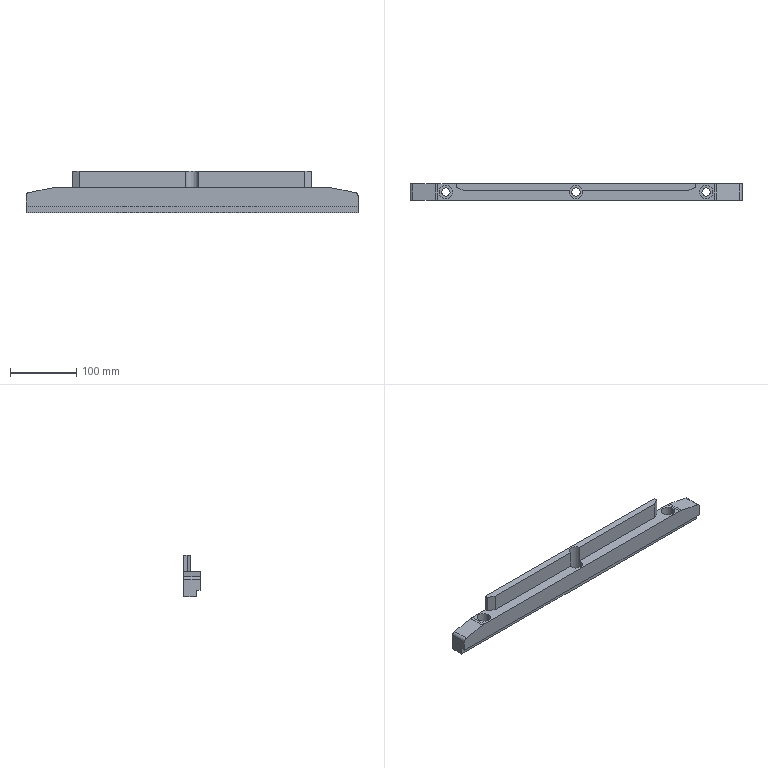NC program | NX | posted with a generic post | part box 500 x 25 x 62.5 mm
Lines 30 to 1063 of 3905:
(ADAPTIVE_MILLING_COPY , TOOL : D12JING)
N52 T21 M6
N54 G54
N56 G17 G0 G90 X258.765 Y-15.498 S9500 M3
N58 G43 Z30. H21
N60 Z-8.
N62 G94 G1 Z-9. F1000.
N64 X257.053 Y-13.023 F3000.
N66 G3 X256.056 Y-12.5 R1.229
N68 G2 X250.891 Y-16.168 R9.884
N70 X243.653 Y-17.311 R27.235
N72 X230.756 Y-17.483 R318.29
N74 G1 X225.881 Y-17.486
N76 X200.156 Y-17.487
N78 X50.756
N80 X50.081 Y-17.49
N82 X49.031 Y-17.492
N84 X48.581
N86 X47.681 Y-17.495
N88 X46.406 Y-17.493
N90 X45.581 Y-17.496
N92 X44.456 Y-17.495
N94 X43.631 Y-17.497
N96 X42.581 Y-17.496
N98 X41.681 Y-17.498
N100 X40.931 Y-17.497
N102 X39.881 Y-17.499
N104 X39.356
N106 X38.681 Y-17.498
N108 X37.856 Y-17.499
N110 X36.806 Y-17.498
N112 X35.981 Y-17.499
N114 X35.006 Y-17.498
N116 X33.956 Y-17.5
N118 X33.131 Y-17.498
N120 X31.931 Y-17.5
N122 X31.031 Y-17.498
N124 X30.206 Y-17.499
N126 X29.006 Y-17.497
N128 X28.181 Y-17.499
N130 X27.056 Y-17.497
N132 X26.081 Y-17.5
N134 X25.106 Y-17.497
N136 X24.056 Y-17.5
N138 X23.156 Y-17.498
N140 X22.256 Y-17.499
N142 X21.206 Y-17.497
N144 X20.231 Y-17.5
N146 X19.256 Y-17.498
N148 X18.206 Y-17.5
N150 X17.306 Y-17.498
N152 X16.406 Y-17.499
N154 X15.431 Y-17.498
N156 X14.756 Y-17.499
N158 X13.706 Y-17.497
N160 X13.256
N162 X12.656 Y-17.499
N164 X11.456 Y-17.497
N166 X10.706 Y-17.498
N168 X9.581 Y-17.497
N170 X8.606 Y-17.499
N172 X7.856 Y-17.498
N174 X6.806 Y-17.499
N176 X6.056 Y-17.498
N178 X4.781 Y-17.5
N180 X3.881 Y-17.498
N182 X3.131 Y-17.499
N184 X1.856 Y-17.497
N186 X1.331 Y-17.496
N188 X0.581 Y-17.498
N190 X-0.619 Y-17.497
N192 X-1.294 Y-17.498
N194 X-2.419 Y-17.497
N196 X-2.869
N198 X-3.469 Y-17.498
N200 X-4.744 Y-17.497
N202 X-5.494 Y-17.498
N204 X-6.544 Y-17.497
N206 X-6.994 Y-17.496
N208 X-7.669 Y-17.497
N210 X-8.944 Y-17.496
N212 X-9.319
N214 X-9.919 Y-17.497
N216 X-11.194 Y-17.496
N218 X-11.719
N220 X-12.394 Y-17.498
N222 X-13.519 Y-17.496
N224 X-14.344 Y-17.498
N226 X-15.619 Y-17.496
N228 X-16.519 Y-17.498
N230 X-17.719 Y-17.496
N232 X-18.394 Y-17.498
N234 X-19.669 Y-17.496
N236 X-20.269
N238 X-20.869 Y-17.497
N240 X-22.069 Y-17.496
N242 X-22.519
N244 X-23.194 Y-17.497
N246 X-24.394 Y-17.496
N248 X-24.844
N250 X-25.444 Y-17.497
N252 X-26.719 Y-17.496
N254 X-27.244 Y-17.495
N256 X-27.919 Y-17.497
N258 X-28.819 Y-17.496
N260 X-29.269
N262 X-30.319 Y-17.499
N264 X-31.294 Y-17.497
N266 X-32.269 Y-17.499
N268 X-33.244 Y-17.497
N270 X-34.219 Y-17.499
N272 X-34.969 Y-17.498
N274 X-36.319 Y-17.5
N276 X-36.769
N278 X-37.444 Y-17.499
N280 X-38.719 Y-17.5
N282 X-39.244 Y-17.501
N284 X-40.069 Y-17.499
N286 X-41.044 Y-17.5
N288 X-42.019 Y-17.498
N290 X-42.844 Y-17.5
N292 X-43.894 Y-17.498
N294 X-44.644 Y-17.499
N296 X-45.844 Y-17.497
N298 X-46.744 Y-17.499
N300 X-47.569 Y-17.498
N302 X-48.694 Y-17.5
N304 X-49.519 Y-17.498
N306 X-50.719 Y-17.5
N308 X-51.619 Y-17.498
N310 X-52.444 Y-17.499
N312 X-53.719 Y-17.497
N314 X-54.694 Y-17.5
N316 X-55.669 Y-17.497
N318 X-56.719 Y-17.5
N320 X-57.694 Y-17.498
N322 X-58.744 Y-17.5
N324 X-59.644 Y-17.498
N326 X-60.469 Y-17.499
N328 X-61.669 Y-17.497
N330 X-62.494 Y-17.499
N332 X-63.694 Y-17.497
N334 X-64.519 Y-17.499
N336 X-65.569 Y-17.497
N338 X-66.319 Y-17.499
N340 X-67.519 Y-17.497
N342 X-68.344 Y-17.499
N344 X-69.619 Y-17.497
N346 X-70.294 Y-17.498
N348 X-71.644 Y-17.497
N350 X-72.169 Y-17.496
N352 X-73.069 Y-17.499
N354 X-73.819 Y-17.498
N356 X-75.169 Y-17.499
N358 X-75.694 Y-17.5
N360 X-76.594 Y-17.498
N362 X-77.344 Y-17.499
N364 X-78.469 Y-17.498
N366 X-79.144
N368 X-79.669 Y-17.499
N370 X-80.494 Y-17.498
N372 X-81.619 Y-17.5
N374 X-82.519 Y-17.498
N376 X-83.269 Y-17.499
N378 X-84.319 Y-17.498
N380 X-84.844
N382 X-85.444 Y-17.499
N384 X-86.569 Y-17.497
N386 X-87.469 Y-17.499
N388 X-88.519 Y-17.497
N390 X-89.569 Y-17.499
N392 X-90.544 Y-17.498
N394 X-91.519 Y-17.499
N396 X-92.494 Y-17.497
N398 X-93.544 Y-17.5
N400 X-94.519 Y-17.498
N402 X-95.494 Y-17.5
N404 X-96.394 Y-17.497
N406 X-97.144 Y-17.499
N408 X-98.194 Y-17.497
N410 X-98.719 Y-17.498
N412 X-99.394 Y-17.499
N414 X-100.219 Y-17.498
N416 X-101.344 Y-17.499
N418 X-102.169 Y-17.498
N420 X-103.369 Y-17.5
N422 X-104.269 Y-17.498
N424 X-105.094 Y-17.499
N426 X-106.219 Y-17.498
N428 X-106.969 Y-17.499
N430 X-108.019 Y-17.498
N432 X-109.069 Y-17.5
N434 X-109.894 Y-17.498
N436 X-111.019 Y-17.5
N438 X-111.769 Y-17.498
N440 X-112.669 Y-17.5
N442 X-113.119
N444 X-114.019 Y-17.498
N446 X-114.919 Y-17.5
N448 X-115.969 Y-17.498
N450 X-116.644 Y-17.499
N452 X-117.769 Y-17.497
N454 X-118.444 Y-17.498
N456 X-118.969 Y-17.499
N458 X-119.794 Y-17.498
N460 X-120.844 Y-17.499
N462 X-121.669 Y-17.498
N464 X-122.644 Y-17.499
N466 X-123.469 Y-17.498
N468 X-124.519 Y-17.5
N470 X-125.269 Y-17.498
N472 X-126.394 Y-17.5
N474 X-126.844
N476 X-127.669 Y-17.498
N478 X-128.794 Y-17.5
N480 X-129.619 Y-17.499
N482 X-130.744 Y-17.5
N484 X-131.494 Y-17.499
N486 X-132.694 Y-17.5
N488 X-133.669 Y-17.498
N490 X-134.419 Y-17.499
N492 X-135.469 Y-17.498
N494 X-135.919 Y-17.497
N496 X-136.819 Y-17.499
N498 X-137.644 Y-17.498
N500 X-138.844 Y-17.5
N502 X-139.819 Y-17.498
N504 X-140.644 Y-17.499
N506 X-141.694 Y-17.498
N508 X-142.369 Y-17.499
N510 X-143.419 Y-17.497
N512 X-143.869
N514 X-144.694 Y-17.499
N516 X-145.819 Y-17.497
N518 X-146.719 Y-17.499
N520 X-147.544 Y-17.498
N522 X-148.744 Y-17.499
N524 X-149.644 Y-17.498
N526 X-150.544 Y-17.499
N528 X-151.444 Y-17.498
N530 X-152.494 Y-17.5
N532 X-153.469 Y-17.498
N534 X-154.369 Y-17.5
N536 X-155.269 Y-17.498
N538 X-156.469 Y-17.5
N540 X-157.369 Y-17.498
N542 X-158.194 Y-17.499
N544 X-159.469 Y-17.497
N546 X-160.294 Y-17.499
N548 X-161.419 Y-17.497
N550 X-162.319 Y-17.499
N552 X-163.144 Y-17.498
N554 X-164.269 Y-17.499
N556 X-165.019 Y-17.498
N558 X-166.219 Y-17.5
N560 X-167.194 Y-17.498
N562 X-168.094 Y-17.5
N564 X-168.994 Y-17.498
N566 X-170.194 Y-17.5
N568 X-171.019 Y-17.498
N570 X-172.219 Y-17.5
N572 X-173.119 Y-17.498
N574 X-173.944 Y-17.499
N576 X-175.144 Y-17.497
N578 X-175.969 Y-17.499
N580 X-177.094 Y-17.497
N582 X-178.069 Y-17.5
N584 X-179.044 Y-17.497
N586 X-179.794 Y-17.498
N588 X-181.144 Y-17.497
N590 X-181.744 Y-17.496
N592 X-182.569 Y-17.498
N594 X-183.469 Y-17.497
N596 X-184.369 Y-17.499
N598 X-185.419 Y-17.497
N600 X-186.244 Y-17.499
N602 X-187.369 Y-17.497
N604 X-188.344 Y-17.499
N606 X-189.094 Y-17.498
N608 X-190.444 Y-17.5
N610 X-191.044 Y-17.501
N612 X-191.944 Y-17.498
N614 X-192.919 Y-17.5
N616 X-193.819 Y-17.498
N618 X-194.644 Y-17.499
N620 X-195.769 Y-17.498
N622 X-196.594 Y-17.499
N624 X-197.569 Y-17.498
N626 X-198.544 Y-17.5
N628 X-199.294 Y-17.499
N630 X-200.419 Y-17.5
N632 X-200.944
N634 X-201.544 Y-17.498
N636 X-202.744 Y-17.5
N638 X-203.569 Y-17.498
N640 X-204.769 Y-17.5
N642 X-205.669 Y-17.498
N644 X-206.494 Y-17.499
N646 X-207.694 Y-17.498
N648 X-208.594 Y-17.5
N650 X-209.419 Y-17.498
N652 X-210.169 Y-17.499
N654 X-210.694 Y-17.5
N656 X-211.444 Y-17.499
N658 X-212.569 Y-17.5
N660 X-213.244 Y-17.499
N662 X-213.694 Y-17.498
N664 X-214.594 Y-17.5
N666 X-215.719 Y-17.497
N668 X-216.394 Y-17.499
N670 X-217.669 Y-17.497
N672 X-218.644 Y-17.5
N674 X-219.394 Y-17.499
N676 X-220.744 Y-17.5
N678 X-221.194
N680 X-221.869 Y-17.499
N682 X-222.994 Y-17.5
N684 X-224.044 Y-17.497
N686 X-225.094 Y-17.5
N688 X-226.069 Y-17.498
N690 X-226.819 Y-17.499
N692 X-227.869 Y-17.497
N694 X-228.244
N696 X-229.219 Y-17.499
N698 X-230.194 Y-17.497
N700 X-231.244 Y-17.5
N702 X-232.219 Y-17.498
N704 X-233.269 Y-17.5
N706 X-234.169 Y-17.498
N708 X-234.994 Y-17.499
N710 X-236.194 Y-17.497
N712 X-236.944 Y-17.499
N714 X-238.219 Y-17.497
N716 G2 X-247.293 Y-17.466 R338.126
N718 X-251.787 Y-15.231 R8.352
N720 G3 X-254.442 Y-12.803 R48.932
N722 X-255.128 Y-12.523 R1.722
N724 G1 X-256.288 Y-12.828
N726 G3 X-257.138 Y-14.315 R1.205
N728 X-256.264 Y-15.161 Z-8.947 R1.241
N730 G1 X-255.197 Y-15.525 Z-8.9
N732 X-254.821 Y-15.652
N734 X-254.451 Y-15.797
N736 G2 X-254.891 Y-18.044 R1.201
N738 G1 X-256.888 Y-18.268
N740 G2 X-258.177 Y-16.749 R1.203
N742 G1 X-257.887 Y-15.724
N744 X-257.233 Y-13.415 Z-9.
N746 G2 X-256.888 Y-12.868 R1.259
N748 X-256.039 Y-12.518 R1.291
N750 X-254.624 Y-12.598 R4.806
N752 X-252.196 Y-14.213 R12.322
N754 G3 X-246.15 Y-16.472 R12.84
N756 X-237.616 Y-16.875 R67.951
N758 G1 X-236.491 Y-16.881
N760 X-234.016 Y-16.889
N762 X-231.541 Y-16.894
N764 X-229.066
N766 X-228.466
N768 X-227.491 Y-16.897
N770 X-226.441 Y-16.896
N772 X-225.991 Y-16.897
N774 X-225.541 Y-16.896
N776 X-225.316 Y-16.897
N778 X-224.041 Y-16.896
N780 X-223.366 Y-16.898
N782 X-222.541 Y-16.896
N784 X-222.016 Y-16.898
N786 X-221.491 Y-16.897
N788 X-221.041 Y-16.898
N790 X-220.291 Y-16.897
N792 X-218.866 Y-16.9
N794 X-218.416 Y-16.899
N796 X-217.216 Y-16.901
N798 X-216.016 Y-16.899
N800 X-215.416 Y-16.9
N802 X-213.841 Y-16.897
N804 X-212.866 Y-16.899
N806 X-212.416
N808 X-210.916 Y-16.901
N810 X-210.016 Y-16.899
N812 X-209.416 Y-16.9
N814 X-208.366 Y-16.898
N816 X-207.016 Y-16.901
N818 X-205.891 Y-16.898
N820 X-205.366 Y-16.899
N822 X-203.716 Y-16.897
N824 X-202.966 Y-16.899
N826 X-202.516 Y-16.898
N828 X-201.991 Y-16.899
N830 X-201.541 Y-16.898
N832 X-200.866 Y-16.9
N834 X-199.741 Y-16.897
N836 X-198.916 Y-16.899
N838 X-198.016 Y-16.897
N840 X-197.041 Y-16.9
N842 X-196.591 Y-16.899
N844 X-192.991 Y-16.902
N846 X-189.391
N848 X-185.791 Y-16.897
N850 X-185.416
N852 X-184.816 Y-16.898
N854 X-184.216 Y-16.896
N856 X-183.691 Y-16.897
N858 X-183.316
N860 X-182.566 Y-16.898
N862 X-181.441 Y-16.896
N864 X-180.391 Y-16.899
N866 X-179.866 Y-16.898
N868 X-178.366 Y-16.9
N870 X-177.316 Y-16.898
N872 X-176.866
N874 X-175.216 Y-16.896
N876 X-174.466 Y-16.898
N878 X-173.866 Y-16.897
N880 X-172.516 Y-16.9
N882 X-171.916 Y-16.898
N884 X-170.491 Y-16.901
N886 X-170.041 Y-16.9
N888 X-166.441 Y-16.902
N890 X-162.841 Y-16.9
N892 X-161.041 Y-16.897
N894 X-160.441 Y-16.898
N896 X-159.916 Y-16.899
N898 X-159.166 Y-16.9
N900 X-157.666 Y-16.897
N902 X-156.691 Y-16.899
N904 X-155.716 Y-16.897
N906 X-154.741 Y-16.9
N908 X-153.691 Y-16.897
N910 X-152.866 Y-16.899
N912 X-151.891 Y-16.897
N914 X-150.991 Y-16.899
N916 X-149.866 Y-16.897
N918 X-149.041 Y-16.899
N920 X-148.516 Y-16.898
N922 X-146.791 Y-16.901
N924 X-146.191 Y-16.899
N926 X-145.516 Y-16.9
N928 X-145.066 Y-16.899
N930 X-144.616 Y-16.9
N932 X-143.866 Y-16.898
N934 X-143.416
N936 X-141.466 Y-16.896
N938 X-141.016 Y-16.897
N940 X-140.566 Y-16.896
N942 X-140.116 Y-16.897
N944 X-139.666 Y-16.896
N946 X-139.066 Y-16.898
N948 X-138.391 Y-16.896
N950 X-137.866 Y-16.898
N952 X-137.341 Y-16.897
N954 X-136.816 Y-16.898
N956 X-136.291
N958 X-135.541 Y-16.899
N960 X-134.191 Y-16.897
N962 X-133.141 Y-16.9
N964 X-131.941 Y-16.897
N966 X-131.116 Y-16.899
N968 X-130.366 Y-16.898
N970 X-128.791 Y-16.901
N972 X-127.891 Y-16.899
N974 X-126.766 Y-16.901
N976 X-125.791 Y-16.898
N978 X-124.816 Y-16.9
N980 X-124.066 Y-16.898
N982 X-123.016 Y-16.9
N984 X-122.116 Y-16.898
N986 X-121.666
N988 X-118.066 Y-16.895
N990 X-114.466
N992 X-110.866 Y-16.899
N994 X-110.116 Y-16.9
N996 X-109.666 Y-16.899
N998 X-109.141 Y-16.9
N1000 X-108.466 Y-16.898
N1002 X-107.341 Y-16.9
N1004 X-106.666 Y-16.899
N1006 X-106.066 Y-16.9
N1008 X-104.491 Y-16.897
N1010 X-103.591 Y-16.899
N1012 X-102.466 Y-16.897
N1014 X-101.641 Y-16.899
N1016 X-101.191 Y-16.898
N1018 X-99.391 Y-16.901
N1020 X-98.791 Y-16.899
N1022 X-98.116 Y-16.9
N1024 X-96.841 Y-16.898
N1026 X-95.866 Y-16.9
N1028 X-94.816 Y-16.897
N1030 X-93.766 Y-16.9
N1032 X-92.791 Y-16.897
N1034 X-92.266 Y-16.898
N1036 X-91.216 Y-16.896
N1038 X-89.791 Y-16.899
N1040 X-89.266
N1042 X-87.466 Y-16.901
N1044 X-86.866 Y-16.899
N1046 X-86.266 Y-16.9
N1048 X-85.816 Y-16.899
N1050 X-85.516 Y-16.9
N1052 X-84.916 Y-16.898
N1054 X-84.241 Y-16.9
N1056 X-82.666 Y-16.897
N1058 X-82.141
N1060 X-81.166 Y-16.896
N1062 X-79.966 Y-16.899
N1064 X-78.766 Y-16.897
N1066 X-78.316 Y-16.898
N1068 X-77.116 Y-16.896
N1070 X-76.666 Y-16.897
N1072 X-75.991 Y-16.896
N1074 X-75.391 Y-16.897
N1076 X-74.641 Y-16.896
N1078 X-73.066 Y-16.899
N1080 X-72.016 Y-16.896
N1082 X-71.416 Y-16.898
N1084 X-70.891 Y-16.897
N1086 X-70.591 Y-16.898
N1088 X-70.066 Y-16.897
N1090 X-69.541 Y-16.898
N1092 X-69.016 Y-16.897
N1094 X-68.641 Y-16.898
N1096 X-67.741 Y-16.896
N1098 X-66.841 Y-16.898
N1100 X-66.316 Y-16.897
N1102 X-64.816 Y-16.9
N1104 X-63.916 Y-16.898
N1106 X-62.716 Y-16.9
N1108 X-61.966 Y-16.898
N1110 X-61.441 Y-16.899
N1112 X-59.941 Y-16.897
N1114 X-59.041 Y-16.899
N1116 X-58.291 Y-16.897
N1118 X-57.391 Y-16.899
N1120 X-55.816 Y-16.896
N1122 X-54.841 Y-16.899
N1124 X-54.316
N1126 X-52.141 Y-16.902
N1128 X-51.691 Y-16.901
N1130 X-51.091
N1132 X-50.641
N1134 X-48.916 Y-16.902
N1136 X-48.166 Y-16.9
N1138 X-47.566 Y-16.901
N1140 X-47.041 Y-16.9
N1142 X-46.666
N1144 X-46.141 Y-16.899
N1146 X-45.691 Y-16.9
N1148 X-44.416 Y-16.897
N1150 X-43.891 Y-16.899
N1152 X-42.466 Y-16.897
N1154 X-41.941 Y-16.898
N1156 X-34.966 Y-16.894
N1158 X-34.516 Y-16.895
N1160 X-33.616 Y-16.894
N1162 X-32.941
N1164 X-32.491 Y-16.895
N1166 X-31.741 Y-16.894
N1168 X-30.691 Y-16.896
N1170 X-29.266 Y-16.894
N1172 X-28.366 Y-16.896
N1174 X-27.016 Y-16.894
N1176 X-26.116 Y-16.897
N1178 X-24.691 Y-16.894
N1180 X-23.791 Y-16.896
N1182 X-22.441 Y-16.894
N1184 X-21.391 Y-16.897
N1186 X-20.041 Y-16.895
N1188 X-18.916 Y-16.898
N1190 X-18.091 Y-16.896
N1192 X-17.566 Y-16.897
N1194 X-16.966 Y-16.896
N1196 X-16.516
N1198 X-15.991
N1200 X-15.391 Y-16.897
N1202 X-13.741 Y-16.894
N1204 X-12.916 Y-16.897
N1206 X-11.566 Y-16.894
N1208 X-10.591 Y-16.897
N1210 X-9.241 Y-16.895
N1212 X-8.266 Y-16.897
N1214 X-6.991 Y-16.895
N1216 X-6.016 Y-16.898
N1218 X-5.266 Y-16.896
N1220 X-3.766 Y-16.899
N1222 X-2.791 Y-16.897
N1224 X-1.816 Y-16.899
N1226 X-0.841 Y-16.897
N1228 X0.734 Y-16.9
N1230 X1.559 Y-16.898
N1232 X2.084 Y-16.899
N1234 X3.809 Y-16.896
N1236 X4.559 Y-16.898
N1238 X5.009
N1240 X6.509 Y-16.901
N1242 X7.259 Y-16.898
N1244 X8.459 Y-16.9
N1246 X9.134 Y-16.898
N1248 X9.659
N1250 X11.309 Y-16.896
N1252 X12.059 Y-16.898
N1254 X13.259 Y-16.896
N1256 X14.009 Y-16.898
N1258 X15.134 Y-16.896
N1260 X15.809 Y-16.898
N1262 X16.709 Y-16.897
N1264 X17.384 Y-16.898
N1266 X19.034 Y-16.896
N1268 X19.934 Y-16.898
N1270 X20.384
N1272 X21.659 Y-16.9
N1274 X22.184 Y-16.899
N1276 X23.759 Y-16.901
N1278 X24.734 Y-16.899
N1280 X25.334 Y-16.9
N1282 X26.609 Y-16.897
N1284 X27.059
N1286 X29.009 Y-16.895
N1288 X29.534 Y-16.897
N1290 X30.434 Y-16.896
N1292 X31.634 Y-16.899
N1294 X32.384 Y-16.897
N1296 X33.509 Y-16.9
N1298 X34.559 Y-16.897
N1300 X35.609 Y-16.899
N1302 X37.184 Y-16.901
N1304 X38.459 Y-16.898
N1306 X38.984 Y-16.899
N1308 X40.559 Y-16.896
N1310 X41.309 Y-16.897
N1312 X41.909 Y-16.896
N1314 X43.109 Y-16.898
N1316 X43.859 Y-16.895
N1318 X44.759 Y-16.897
N1320 X46.484 Y-16.892
N1322 X47.084 Y-16.893
N1324 X49.184 Y-16.888
N1326 X50.009 Y-16.889
N1328 X50.534 Y-16.888
N1330 X51.284 Y-16.889
N1332 X51.809 Y-16.888
N1334 X52.634 Y-16.889
N1336 X53.159 Y-16.888
N1338 X53.984 Y-16.889
N1340 X54.509 Y-16.888
N1342 X55.334 Y-16.889
N1344 X55.859 Y-16.888
N1346 X56.684 Y-16.889
N1348 X57.209 Y-16.888
N1350 X57.959 Y-16.889
N1352 X58.484 Y-16.888
N1354 X59.309 Y-16.889
N1356 X59.834 Y-16.888
N1358 X60.659 Y-16.889
N1360 X61.184 Y-16.888
N1362 X62.009 Y-16.889
N1364 X62.534 Y-16.888
N1366 X63.359 Y-16.889
N1368 X63.884 Y-16.888
N1370 X64.709 Y-16.889
N1372 X65.234 Y-16.888
N1374 X65.984 Y-16.889
N1376 X66.509 Y-16.888
N1378 X67.334 Y-16.889
N1380 X67.859 Y-16.888
N1382 X68.684 Y-16.889
N1384 X69.209 Y-16.888
N1386 X70.034 Y-16.889
N1388 X70.559 Y-16.888
N1390 X71.384 Y-16.889
N1392 X71.909 Y-16.888
N1394 X72.659 Y-16.889
N1396 X73.184 Y-16.888
N1398 X74.009 Y-16.889
N1400 X74.534 Y-16.888
N1402 X75.359 Y-16.889
N1404 X75.884 Y-16.888
N1406 X76.709 Y-16.889
N1408 X77.234 Y-16.888
N1410 X78.059 Y-16.889
N1412 X78.584 Y-16.888
N1414 X79.409 Y-16.889
N1416 X79.934 Y-16.888
N1418 X80.684 Y-16.889
N1420 X81.209 Y-16.888
N1422 X82.034 Y-16.889
N1424 X82.559 Y-16.888
N1426 X83.384 Y-16.889
N1428 X83.909 Y-16.888
N1430 X84.734 Y-16.889
N1432 X85.259 Y-16.888
N1434 X86.084 Y-16.889
N1436 X86.609 Y-16.888
N1438 X87.359 Y-16.889
N1440 X87.884 Y-16.888
N1442 X88.709 Y-16.889
N1444 X89.234 Y-16.888
N1446 X90.059 Y-16.889
N1448 X90.584 Y-16.888
N1450 X91.409 Y-16.889
N1452 X91.934 Y-16.888
N1454 X92.759 Y-16.889
N1456 X93.284 Y-16.888
N1458 X94.109 Y-16.889
N1460 X94.634 Y-16.888
N1462 X95.384 Y-16.889
N1464 X95.909 Y-16.888
N1466 X96.734 Y-16.889
N1468 X97.259 Y-16.888
N1470 X98.084 Y-16.889
N1472 X98.609 Y-16.888
N1474 X99.434 Y-16.889
N1476 X99.959 Y-16.888
N1478 X100.784 Y-16.889
N1480 X101.309 Y-16.888
N1482 X102.134 Y-16.889
N1484 X102.734 Y-16.887
N1486 X103.634 Y-16.889
N1488 X104.159 Y-16.888
N1490 X104.984 Y-16.889
N1492 X105.509 Y-16.888
N1494 X106.334 Y-16.889
N1496 X106.934 Y-16.887
N1498 X107.834 Y-16.889
N1500 X108.359 Y-16.888
N1502 X109.184 Y-16.889
N1504 X109.709 Y-16.888
N1506 X110.534 Y-16.889
N1508 X111.134 Y-16.887
N1510 X112.034 Y-16.889
N1512 X112.559 Y-16.888
N1514 X113.384 Y-16.889
N1516 X113.909 Y-16.888
N1518 X114.734 Y-16.889
N1520 X115.334 Y-16.887
N1522 X116.234 Y-16.889
N1524 X116.759 Y-16.888
N1526 X117.584 Y-16.889
N1528 X118.109 Y-16.888
N1530 X118.934 Y-16.889
N1532 X119.534 Y-16.887
N1534 X120.434 Y-16.889
N1536 X120.959 Y-16.888
N1538 X121.784 Y-16.889
N1540 X122.309 Y-16.888
N1542 X123.134 Y-16.889
N1544 X123.734 Y-16.887
N1546 X124.634 Y-16.889
N1548 X125.159 Y-16.888
N1550 X125.984 Y-16.889
N1552 X126.509 Y-16.888
N1554 X127.334 Y-16.889
N1556 X127.934 Y-16.887
N1558 X128.834 Y-16.889
N1560 X129.358 Y-16.888
N1562 X130.183 Y-16.889
N1564 X130.708 Y-16.888
N1566 X131.533 Y-16.889
N1568 X132.133 Y-16.887
N1570 X133.033 Y-16.889
N1572 X133.558 Y-16.888
N1574 X134.383 Y-16.889
N1576 X134.908 Y-16.888
N1578 X135.733 Y-16.889
N1580 X136.333 Y-16.887
N1582 X137.233 Y-16.889
N1584 X137.758 Y-16.888
N1586 X138.583 Y-16.889
N1588 X139.108 Y-16.888
N1590 X139.933 Y-16.889
N1592 X140.533 Y-16.887
N1594 X141.433 Y-16.889
N1596 X141.958 Y-16.888
N1598 X142.783 Y-16.889
N1600 X143.308 Y-16.888
N1602 X144.133 Y-16.889
N1604 X144.733 Y-16.887
N1606 X145.633 Y-16.889
N1608 X146.158 Y-16.888
N1610 X146.983 Y-16.889
N1612 X147.508 Y-16.888
N1614 X148.333 Y-16.889
N1616 X148.933 Y-16.887
N1618 X149.833 Y-16.889
N1620 X150.358 Y-16.888
N1622 X151.183 Y-16.889
N1624 X151.708 Y-16.888
N1626 X152.533 Y-16.889
N1628 X153.058 Y-16.888
N1630 X153.808 Y-16.889
N1632 X154.333 Y-16.888
N1634 X155.158 Y-16.889
N1636 X155.683 Y-16.888
N1638 X156.508 Y-16.889
N1640 X157.033 Y-16.888
N1642 X157.858 Y-16.889
N1644 X158.383 Y-16.888
N1646 X159.208 Y-16.889
N1648 X159.733 Y-16.888
N1650 X160.483 Y-16.889
N1652 X161.008 Y-16.888
N1654 X161.833 Y-16.889
N1656 X162.358 Y-16.888
N1658 X163.183 Y-16.889
N1660 X163.708 Y-16.888
N1662 X164.533 Y-16.889
N1664 X165.058 Y-16.888
N1666 X165.883 Y-16.889
N1668 X166.408 Y-16.888
N1670 X167.233 Y-16.889
N1672 X167.758 Y-16.888
N1674 X168.508 Y-16.889
N1676 X169.033 Y-16.888
N1678 X169.858 Y-16.889
N1680 X170.383 Y-16.888
N1682 X171.208 Y-16.889
N1684 X171.733 Y-16.888
N1686 X172.558 Y-16.889
N1688 X173.083 Y-16.888
N1690 X173.908 Y-16.889
N1692 X174.433 Y-16.888
N1694 X175.183 Y-16.889
N1696 X175.708 Y-16.888
N1698 X176.533 Y-16.889
N1700 X177.058 Y-16.888
N1702 X177.883 Y-16.889
N1704 X178.408 Y-16.888
N1706 X179.233 Y-16.889
N1708 X179.758 Y-16.888
N1710 X180.583 Y-16.889
N1712 X181.108 Y-16.888
N1714 X181.933 Y-16.889
N1716 X182.458 Y-16.888
N1718 X183.208 Y-16.889
N1720 X183.733 Y-16.888
N1722 X184.558 Y-16.889
N1724 X185.083 Y-16.888
N1726 X185.908 Y-16.889
N1728 X186.433 Y-16.888
N1730 X187.258 Y-16.889
N1732 X187.783 Y-16.888
N1734 X188.608 Y-16.889
N1736 X189.133 Y-16.888
N1738 X189.883 Y-16.889
N1740 X190.408 Y-16.888
N1742 X191.233 Y-16.889
N1744 X191.758 Y-16.888
N1746 X192.583 Y-16.889
N1748 X193.108 Y-16.888
N1750 X193.933 Y-16.889
N1752 X194.458 Y-16.888
N1754 X195.283 Y-16.889
N1756 X195.808 Y-16.888
N1758 X196.633 Y-16.889
N1760 X197.158 Y-16.888
N1762 X197.908 Y-16.889
N1764 X198.433 Y-16.888
N1766 X199.258 Y-16.889
N1768 X199.783 Y-16.888
N1770 X200.608 Y-16.889
N1772 X201.133 Y-16.888
N1774 X201.958 Y-16.889
N1776 X202.483 Y-16.888
N1778 X203.308 Y-16.889
N1780 X203.833 Y-16.888
N1782 X204.583 Y-16.889
N1784 X205.108 Y-16.888
N1786 X205.933 Y-16.889
N1788 X206.458 Y-16.888
N1790 X207.283 Y-16.889
N1792 X207.808 Y-16.888
N1794 X208.633 Y-16.889
N1796 X209.158 Y-16.888
N1798 X209.983 Y-16.889
N1800 X210.508 Y-16.888
N1802 X211.258 Y-16.889
N1804 X211.783 Y-16.887
N1806 X212.608 Y-16.889
N1808 X213.133 Y-16.888
N1810 X213.958 Y-16.889
N1812 X214.483 Y-16.888
N1814 X215.233 Y-16.889
N1816 X215.758 Y-16.887
N1818 X216.583 Y-16.889
N1820 X217.108 Y-16.887
N1822 X217.858 Y-16.889
N1824 X218.383 Y-16.887
N1826 X219.208 Y-16.889
N1828 X219.808 Y-16.887
N1830 X220.633 Y-16.889
N1832 X221.233 Y-16.887
N1834 X222.058 Y-16.888
N1836 X222.658 Y-16.887
N1838 X223.408 Y-16.888
N1840 X224.008 Y-16.887
N1842 X224.683 Y-16.888
N1844 X225.358 Y-16.886
N1846 X226.033 Y-16.887
N1848 X226.783 Y-16.885
N1850 X227.383 Y-16.886
N1852 X228.283 Y-16.884
N1854 X228.733
N1856 X230.008 Y-16.881
N1858 X230.383 Y-16.882
N1860 G3 X244.029 Y-16.641 R234.988
N1862 X250.552 Y-15.363 R21.345
N1864 X254.118 Y-13.166 R17.565
N1866 G2 X255.444 Y-12.501 R3.071
N1868 X256.084 Y-12.684 R1.269
N1870 G1 X256.637 Y-13.021
N1872 X257.174 Y-13.383
N1874 G2 X256.367 Y-15.499 R1.213
N1876 G1 Z-6.
N1878 G0 Z30.
N1880 X-255.909 Y-15.529
N1882 Z-8.
N1884 G1 Z-9. F1000.
N1886 G2 X-256.561 Y-13.295 R1.213 F3000.
N1888 G1 X-256.03 Y-12.954
N1890 X-255.491 Y-12.627
N1892 X-255.245 Y-12.55
N1894 X-254.989 Y-12.519
N1896 G2 X-253.098 Y-13.168 R3.787
N1898 G3 X-243.462 Y-15.986 R22.571
N1900 X-232.519 Y-16.28 R143.93
N1902 G1 X-231.019 Y-16.284
N1904 X-230.419 Y-16.287
N1906 X-229.069 Y-16.288
N1908 X-228.544 Y-16.291
N1910 X-228.019 Y-16.292
N1912 X-227.569
N1914 X-226.669
N1916 X-225.844 Y-16.294
N1918 X-225.169
N1920 X-224.344 Y-16.296
N1922 X-223.744 Y-16.295
N1924 X-223.369 Y-16.296
N1926 X-222.769
N1928 X-222.394
N1930 X-222.019
N1932 X-221.269 Y-16.298
N1934 X-220.594 Y-16.297
N1936 X-219.619 Y-16.3
N1938 X-218.719 Y-16.298
N1940 X-217.669 Y-16.3
N1942 X-216.319 Y-16.297
N1944 X-215.269 Y-16.299
N1946 X-214.894 Y-16.298
N1948 X-213.394 Y-16.302
N1950 X-212.644 Y-16.3
N1952 X-211.369 Y-16.301
N1954 X-210.77 Y-16.299
N1956 X-209.645 Y-16.301
N1958 X-208.22 Y-16.298
N1960 X-207.62 Y-16.3
N1962 X-206.27 Y-16.297
N1964 X-205.595 Y-16.298
N1966 X-205.145 Y-16.297
N1968 X-204.245 Y-16.299
N1970 X-203.72
N1972 X-203.195 Y-16.3
N1974 X-202.145 Y-16.297
N1976 X-201.245 Y-16.299
N1978 X-200.42 Y-16.297
N1980 X-199.145 Y-16.3
N1982 X-198.77 Y-16.299
N1984 X-197.42 Y-16.302
N1986 X-196.97 Y-16.301
N1988 X-196.07 Y-16.303
N1990 X-195.545 Y-16.302
N1992 X-194.795 Y-16.303
N1994 X-194.195 Y-16.302
N1996 X-193.595 Y-16.303
N1998 X-192.845 Y-16.302
N2000 X-192.32 Y-16.303
N2002 X-191.345 Y-16.301
N2004 X-190.895 Y-16.302
N2006 X-189.395 Y-16.298
N2008 X-189.02 Y-16.299
N2010 X-187.82 Y-16.296
N2012 X-187.295 Y-16.297
N2014 X-186.62 Y-16.296
N2016 X-186.02 Y-16.297
N2018 X-185.645 Y-16.296
N2020 X-184.895 Y-16.298
N2022 X-183.845 Y-16.296
N2024 X-182.72 Y-16.298
N2026 X-182.12 Y-16.297
N2028 X-180.845 Y-16.3
N2030 X-179.945 Y-16.299
N2032 X-179.495
N2034 X-178.97 Y-16.297
N2036 X-178.52 Y-16.298
N2038 X-177.62 Y-16.296
N2040 X-177.095 Y-16.298
N2042 X-176.195 Y-16.296
N2044 X-174.995 Y-16.299
N2046 X-174.095 Y-16.298
N2048 X-172.97 Y-16.3
N2050 X-172.295 Y-16.299
N2052 X-171.545 Y-16.301
N2054 X-170.945 Y-16.3
N2056 X-170.27 Y-16.302
N2058 X-169.52 Y-16.3
N2060 X-168.92 Y-16.302
N2062 X-167.945 Y-16.3
N2064 X-167.495 Y-16.301
N2066 X-166.145 Y-16.299
N2068 X-165.77 Y-16.3
N2070 X-163.595 Y-16.296
N2072 X-162.395 Y-16.299
N2074 X-162.02 Y-16.298
N2076 X-161.495 Y-16.3
N2078 X-159.845 Y-16.297
N2080 X-159.02 Y-16.299
N2082 X-157.97 Y-16.297
N2084 X-157.145 Y-16.299
N2086 X-155.945 Y-16.297
N2088 X-155.195 Y-16.299
N2090 X-154.67 Y-16.298
N2092 X-153.32 Y-16.3
N2094 X-152.345 Y-16.298
N2096 X-151.07 Y-16.3
N2098 X-150.695 Y-16.299
N2100 X-149.27 Y-16.302
N2102 X-148.445 Y-16.3
N2104 X-147.77 Y-16.301
N2106 X-147.395 Y-16.3
N2108 X-146.945 Y-16.301
N2110 X-146.27 Y-16.299
N2112 X-145.82 Y-16.3